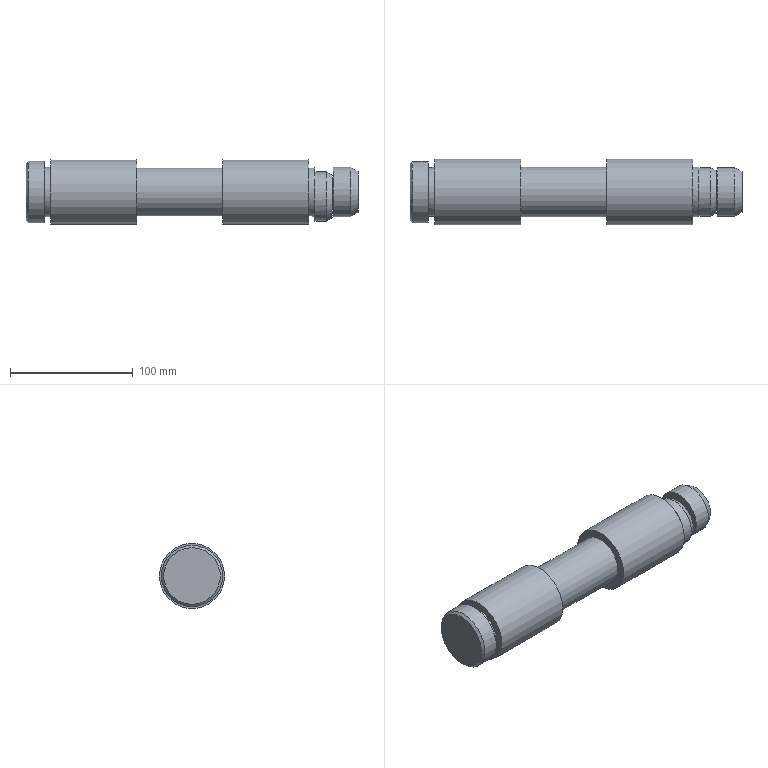Part | NX | features solid 2 | 1 solid | 33 faces | box 270 x 53 x 53 mm | volume 475072 mm3 | plane 14 | cylinder 12 | cone 7 | commonest cylinder face diameters 40 x5 53 x2 16 x1 16.2 x1 20 x1 27 x1
STEP:
#1=CARTESIAN_POINT('',(-925.,645.,-195.));
#2=VERTEX_POINT('',#1);
#3=CARTESIAN_POINT('',(-925.,625.,-195.));
#4=DIRECTION('',(1.,0.,0.));
#5=DIRECTION('',(0.,1.,0.));
#6=AXIS2_PLACEMENT_3D('',#3,#4,#5);
#7=CIRCLE('',#6,20.);
#8=EDGE_CURVE('',#2,#2,#7,.T.);
#9=ORIENTED_EDGE('',*,*,#8,.T.);
#10=EDGE_LOOP('',(#9));
#11=FACE_BOUND('',#10,.T.);
#12=CARTESIAN_POINT('',(-920.001,644.919,-196.8));
#13=VERTEX_POINT('',#12);
#14=CARTESIAN_POINT('',(-920.001,605.081,-196.8));
#15=VERTEX_POINT('',#14);
#16=CARTESIAN_POINT('',(-920.001,625.,-195.));
#17=DIRECTION('',(-1.,0.,0.));
#18=DIRECTION('',(0.,0.,1.));
#19=AXIS2_PLACEMENT_3D('',#16,#17,#18);
#20=CIRCLE('',#19,20.);
#21=EDGE_CURVE('',#13,#15,#20,.T.);
#22=ORIENTED_EDGE('',*,*,#21,.T.);
#23=CARTESIAN_POINT('',(-920.001,625.,-195.));
#24=DIRECTION('',(-1.,0.,0.));
#25=DIRECTION('',(0.,0.,1.));
#26=AXIS2_PLACEMENT_3D('',#23,#24,#25);
#27=CIRCLE('',#26,20.);
#28=EDGE_CURVE('',#15,#13,#27,.T.);
#29=ORIENTED_EDGE('',*,*,#28,.T.);
#30=EDGE_LOOP('',(#22,#29));
#31=FACE_BOUND('',#30,.T.);
#32=CARTESIAN_POINT('',(-1140.001,625.,-195.));
#33=DIRECTION('',(1.,0.,0.));
#34=DIRECTION('',(0.,0.,1.));
#35=AXIS2_PLACEMENT_3D('',#32,#33,#34);
#36=CYLINDRICAL_SURFACE('',#35,20.);
#37=ADVANCED_FACE('',(#11,#31),#36,.T.);
#38=CARTESIAN_POINT('',(-920.001,625.,-198.6));
#39=DIRECTION('',(-1.,0.,0.));
#40=DIRECTION('',(0.,-1.,0.));
#41=AXIS2_PLACEMENT_3D('',#38,#39,#40);
#42=CIRCLE('',#41,20.);
#43=EDGE_CURVE('',#15,#13,#42,.T.);
#44=ORIENTED_EDGE('',*,*,#43,.T.);
#45=ORIENTED_EDGE('',*,*,#28,.F.);
#46=EDGE_LOOP('',(#44,#45));
#47=FACE_BOUND('',#46,.T.);
#48=CARTESIAN_POINT('',(-920.001,625.,-195.));
#49=DIRECTION('',(1.,0.,0.));
#50=DIRECTION('',(0.,0.,1.));
#51=AXIS2_PLACEMENT_3D('',#48,#49,#50);
#52=PLANE('',#51);
#53=ADVANCED_FACE('',(#47),#52,.T.);
#54=CARTESIAN_POINT('',(-910.501,625.,-178.6));
#55=VERTEX_POINT('',#54);
#56=CARTESIAN_POINT('',(-910.501,625.,-198.6));
#57=DIRECTION('',(-1.,0.,0.));
#58=DIRECTION('',(0.,0.,1.));
#59=AXIS2_PLACEMENT_3D('',#56,#57,#58);
#60=CIRCLE('',#59,20.);
#61=EDGE_CURVE('',#55,#55,#60,.T.);
#62=ORIENTED_EDGE('',*,*,#61,.T.);
#63=EDGE_LOOP('',(#62));
#64=FACE_BOUND('',#63,.T.);
#65=CARTESIAN_POINT('',(-920.001,625.,-198.6));
#66=DIRECTION('',(-1.,0.,0.));
#67=DIRECTION('',(0.,0.,1.));
#68=AXIS2_PLACEMENT_3D('',#65,#66,#67);
#69=CIRCLE('',#68,20.);
#70=EDGE_CURVE('',#13,#15,#69,.T.);
#71=ORIENTED_EDGE('',*,*,#70,.F.);
#72=ORIENTED_EDGE('',*,*,#43,.F.);
#73=EDGE_LOOP('',(#71,#72));
#74=FACE_BOUND('',#73,.T.);
#75=CARTESIAN_POINT('',(-906.001,625.,-198.6));
#76=DIRECTION('',(-1.,0.,0.));
#77=DIRECTION('',(0.,0.,-1.));
#78=AXIS2_PLACEMENT_3D('',#75,#76,#77);
#79=CYLINDRICAL_SURFACE('',#78,20.);
#80=ADVANCED_FACE('',(#64,#74),#79,.T.);
#81=CARTESIAN_POINT('',(-906.001,622.282,-185.376));
#82=VERTEX_POINT('',#81);
#83=CARTESIAN_POINT('',(-906.001,627.718,-185.376));
#84=VERTEX_POINT('',#83);
#85=CARTESIAN_POINT('',(-906.001,625.,-195.));
#86=DIRECTION('',(-1.,0.,0.));
#87=DIRECTION('',(0.,1.,0.));
#88=AXIS2_PLACEMENT_3D('',#85,#86,#87);
#89=CIRCLE('',#88,10.);
#90=EDGE_CURVE('',#82,#84,#89,.T.);
#91=ORIENTED_EDGE('',*,*,#90,.T.);
#92=CARTESIAN_POINT('',(-906.001,625.,-198.6));
#93=DIRECTION('',(-1.,0.,0.));
#94=DIRECTION('',(0.,0.,1.));
#95=AXIS2_PLACEMENT_3D('',#92,#93,#94);
#96=CIRCLE('',#95,13.5);
#97=EDGE_CURVE('',#84,#82,#96,.T.);
#98=ORIENTED_EDGE('',*,*,#97,.T.);
#99=EDGE_LOOP('',(#91,#98));
#100=FACE_BOUND('',#99,.T.);
#101=CARTESIAN_POINT('',(-906.001,625.,-181.198));
#102=VERTEX_POINT('',#101);
#103=CARTESIAN_POINT('',(-906.001,625.,-198.6));
#104=DIRECTION('',(1.,0.,0.));
#105=DIRECTION('',(0.,0.,1.));
#106=AXIS2_PLACEMENT_3D('',#103,#104,#105);
#107=CIRCLE('',#106,17.402);
#108=EDGE_CURVE('',#102,#102,#107,.T.);
#109=ORIENTED_EDGE('',*,*,#108,.T.);
#110=EDGE_LOOP('',(#109));
#111=FACE_BOUND('',#110,.T.);
#112=CARTESIAN_POINT('',(-906.001,625.,-198.6));
#113=DIRECTION('',(-1.,0.,0.));
#114=DIRECTION('',(0.,0.,-1.));
#115=AXIS2_PLACEMENT_3D('',#112,#113,#114);
#116=PLANE('',#115);
#117=ADVANCED_FACE('',(#100,#111),#116,.F.);
#118=ORIENTED_EDGE('',*,*,#70,.T.);
#119=ORIENTED_EDGE('',*,*,#21,.F.);
#120=EDGE_LOOP('',(#118,#119));
#121=FACE_BOUND('',#120,.T.);
#122=CARTESIAN_POINT('',(-920.001,625.,-198.6));
#123=DIRECTION('',(-1.,0.,0.));
#124=DIRECTION('',(0.,0.,-1.));
#125=AXIS2_PLACEMENT_3D('',#122,#123,#124);
#126=PLANE('',#125);
#127=ADVANCED_FACE('',(#121),#126,.T.);
#128=ORIENTED_EDGE('',*,*,#108,.F.);
#129=EDGE_LOOP('',(#128));
#130=FACE_BOUND('',#129,.T.);
#131=ORIENTED_EDGE('',*,*,#61,.F.);
#132=EDGE_LOOP('',(#131));
#133=FACE_BOUND('',#132,.T.);
#134=CARTESIAN_POINT('',(-910.501,625.,-198.6));
#135=DIRECTION('',(-1.,0.,0.));
#136=DIRECTION('',(0.,0.,-1.));
#137=AXIS2_PLACEMENT_3D('',#134,#135,#136);
#138=CONICAL_SURFACE('',#137,20.,0.5236);
#139=ADVANCED_FACE('',(#130,#133),#138,.T.);
#140=CARTESIAN_POINT('',(-919.201,622.282,-185.376));
#141=VERTEX_POINT('',#140);
#142=CARTESIAN_POINT('',(-912.601,622.282,-185.376));
#143=DIRECTION('',(1.,0.,0.));
#144=VECTOR('',#143,1000.);
#145=LINE('',#142,#144);
#146=EDGE_CURVE('',#141,#82,#145,.T.);
#147=ORIENTED_EDGE('',*,*,#146,.T.);
#148=ORIENTED_EDGE('',*,*,#97,.F.);
#149=CARTESIAN_POINT('',(-919.201,627.718,-185.376));
#150=VERTEX_POINT('',#149);
#151=CARTESIAN_POINT('',(-912.601,627.718,-185.376));
#152=DIRECTION('',(-1.,0.,0.));
#153=VECTOR('',#152,1000.);
#154=LINE('',#151,#153);
#155=EDGE_CURVE('',#84,#150,#154,.T.);
#156=ORIENTED_EDGE('',*,*,#155,.T.);
#157=CARTESIAN_POINT('',(-919.201,625.,-198.6));
#158=DIRECTION('',(-1.,0.,0.));
#159=DIRECTION('',(0.,0.,1.));
#160=AXIS2_PLACEMENT_3D('',#157,#158,#159);
#161=CIRCLE('',#160,13.5);
#162=EDGE_CURVE('',#150,#141,#161,.T.);
#163=ORIENTED_EDGE('',*,*,#162,.T.);
#164=EDGE_LOOP('',(#147,#148,#156,#163));
#165=FACE_BOUND('',#164,.T.);
#166=CARTESIAN_POINT('',(-906.001,625.,-198.6));
#167=DIRECTION('',(-1.,0.,0.));
#168=DIRECTION('',(0.,0.,-1.));
#169=AXIS2_PLACEMENT_3D('',#166,#167,#168);
#170=CYLINDRICAL_SURFACE('',#169,13.5);
#171=ADVANCED_FACE('',(#165),#170,.F.);
#172=CARTESIAN_POINT('',(-920.001,610.7,-198.6));
#173=VERTEX_POINT('',#172);
#174=CARTESIAN_POINT('',(-920.001,625.,-198.6));
#175=DIRECTION('',(1.,0.,0.));
#176=DIRECTION('',(0.,-1.,0.));
#177=AXIS2_PLACEMENT_3D('',#174,#175,#176);
#178=CIRCLE('',#177,14.3);
#179=EDGE_CURVE('',#173,#173,#178,.T.);
#180=ORIENTED_EDGE('',*,*,#179,.F.);
#181=EDGE_LOOP('',(#180));
#182=FACE_BOUND('',#181,.T.);
#183=ORIENTED_EDGE('',*,*,#162,.F.);
#184=CARTESIAN_POINT('',(-919.201,622.282,-185.376));
#185=CARTESIAN_POINT('',(-919.334,624.058,-184.875));
#186=CARTESIAN_POINT('',(-919.334,625.942,-184.875));
#187=CARTESIAN_POINT('',(-919.201,627.718,-185.376));
#188=B_SPLINE_CURVE_WITH_KNOTS('',3,(#184,#185,#186,#187),.UNSPECIFIED.,.F.,.F.,(4,4),(0.,0.005472),.UNSPECIFIED.);
#189=EDGE_CURVE('',#141,#150,#188,.T.);
#190=ORIENTED_EDGE('',*,*,#189,.F.);
#191=EDGE_LOOP('',(#183,#190));
#192=FACE_BOUND('',#191,.T.);
#193=CARTESIAN_POINT('',(-919.201,625.,-198.6));
#194=DIRECTION('',(-1.,0.,0.));
#195=DIRECTION('',(0.,0.,-1.));
#196=AXIS2_PLACEMENT_3D('',#193,#194,#195);
#197=CONICAL_SURFACE('',#196,13.5,0.7854);
#198=ADVANCED_FACE('',(#182,#192),#197,.F.);
#199=CARTESIAN_POINT('',(-920.001,625.,-185.));
#200=VERTEX_POINT('',#199);
#201=CARTESIAN_POINT('',(-920.001,625.,-195.));
#202=DIRECTION('',(1.,0.,0.));
#203=DIRECTION('',(0.,0.,1.));
#204=AXIS2_PLACEMENT_3D('',#201,#202,#203);
#205=CIRCLE('',#204,10.);
#206=EDGE_CURVE('',#200,#200,#205,.T.);
#207=ORIENTED_EDGE('',*,*,#206,.T.);
#208=EDGE_LOOP('',(#207));
#209=FACE_BOUND('',#208,.T.);
#210=CARTESIAN_POINT('',(-905.001,635.,-195.));
#211=VERTEX_POINT('',#210);
#212=CARTESIAN_POINT('',(-905.001,625.,-195.));
#213=DIRECTION('',(-1.,0.,0.));
#214=DIRECTION('',(0.,1.,0.));
#215=AXIS2_PLACEMENT_3D('',#212,#213,#214);
#216=CIRCLE('',#215,10.);
#217=EDGE_CURVE('',#211,#211,#216,.T.);
#218=ORIENTED_EDGE('',*,*,#217,.T.);
#219=EDGE_LOOP('',(#218));
#220=FACE_BOUND('',#219,.T.);
#221=ORIENTED_EDGE('',*,*,#146,.F.);
#222=ORIENTED_EDGE('',*,*,#189,.T.);
#223=ORIENTED_EDGE('',*,*,#155,.F.);
#224=ORIENTED_EDGE('',*,*,#90,.F.);
#225=EDGE_LOOP('',(#221,#222,#223,#224));
#226=FACE_BOUND('',#225,.T.);
#227=CARTESIAN_POINT('',(-920.001,625.,-195.));
#228=DIRECTION('',(1.,0.,0.));
#229=DIRECTION('',(0.,0.,1.));
#230=AXIS2_PLACEMENT_3D('',#227,#228,#229);
#231=CYLINDRICAL_SURFACE('',#230,10.);
#232=ADVANCED_FACE('',(#209,#220,#226),#231,.T.);
#233=ORIENTED_EDGE('',*,*,#179,.T.);
#234=EDGE_LOOP('',(#233));
#235=FACE_BOUND('',#234,.T.);
#236=ORIENTED_EDGE('',*,*,#206,.F.);
#237=EDGE_LOOP('',(#236));
#238=FACE_BOUND('',#237,.T.);
#239=CARTESIAN_POINT('',(-920.001,625.,-195.));
#240=DIRECTION('',(1.,0.,0.));
#241=DIRECTION('',(0.,0.,1.));
#242=AXIS2_PLACEMENT_3D('',#239,#240,#241);
#243=PLANE('',#242);
#244=ADVANCED_FACE('',(#235,#238),#243,.T.);
#245=ORIENTED_EDGE('',*,*,#8,.F.);
#246=EDGE_LOOP('',(#245));
#247=FACE_BOUND('',#246,.T.);
#248=CARTESIAN_POINT('',(-925.,651.5,-195.));
#249=VERTEX_POINT('',#248);
#250=CARTESIAN_POINT('',(-925.,625.,-195.));
#251=DIRECTION('',(1.,0.,0.));
#252=DIRECTION('',(0.,1.,0.));
#253=AXIS2_PLACEMENT_3D('',#250,#251,#252);
#254=CIRCLE('',#253,26.5);
#255=EDGE_CURVE('',#249,#249,#254,.T.);
#256=ORIENTED_EDGE('',*,*,#255,.T.);
#257=EDGE_LOOP('',(#256));
#258=FACE_BOUND('',#257,.T.);
#259=CARTESIAN_POINT('',(-925.,625.,-195.));
#260=DIRECTION('',(-1.,0.,0.));
#261=DIRECTION('',(0.,0.,1.));
#262=AXIS2_PLACEMENT_3D('',#259,#260,#261);
#263=PLANE('',#262);
#264=ADVANCED_FACE('',(#247,#258),#263,.F.);
#265=CARTESIAN_POINT('',(-995.,645.,-195.));
#266=VERTEX_POINT('',#265);
#267=CARTESIAN_POINT('',(-995.,625.,-195.));
#268=DIRECTION('',(-1.,0.,0.));
#269=DIRECTION('',(0.,1.,0.));
#270=AXIS2_PLACEMENT_3D('',#267,#268,#269);
#271=CIRCLE('',#270,20.);
#272=EDGE_CURVE('',#266,#266,#271,.T.);
#273=ORIENTED_EDGE('',*,*,#272,.F.);
#274=EDGE_LOOP('',(#273));
#275=FACE_BOUND('',#274,.T.);
#276=CARTESIAN_POINT('',(-995.,651.5,-195.));
#277=VERTEX_POINT('',#276);
#278=CARTESIAN_POINT('',(-995.,625.,-195.));
#279=DIRECTION('',(1.,0.,0.));
#280=DIRECTION('',(0.,1.,0.));
#281=AXIS2_PLACEMENT_3D('',#278,#279,#280);
#282=CIRCLE('',#281,26.5);
#283=EDGE_CURVE('',#277,#277,#282,.T.);
#284=ORIENTED_EDGE('',*,*,#283,.F.);
#285=EDGE_LOOP('',(#284));
#286=FACE_BOUND('',#285,.T.);
#287=CARTESIAN_POINT('',(-995.,625.,-195.));
#288=DIRECTION('',(-1.,0.,0.));
#289=DIRECTION('',(0.,0.,1.));
#290=AXIS2_PLACEMENT_3D('',#287,#288,#289);
#291=PLANE('',#290);
#292=ADVANCED_FACE('',(#275,#286),#291,.T.);
#293=ORIENTED_EDGE('',*,*,#255,.F.);
#294=EDGE_LOOP('',(#293));
#295=FACE_BOUND('',#294,.T.);
#296=ORIENTED_EDGE('',*,*,#283,.T.);
#297=EDGE_LOOP('',(#296));
#298=FACE_BOUND('',#297,.T.);
#299=CARTESIAN_POINT('',(-995.,625.,-195.));
#300=DIRECTION('',(1.,0.,0.));
#301=DIRECTION('',(0.,0.,-1.));
#302=AXIS2_PLACEMENT_3D('',#299,#300,#301);
#303=CYLINDRICAL_SURFACE('',#302,26.5);
#304=ADVANCED_FACE('',(#295,#298),#303,.T.);
#305=CARTESIAN_POINT('',(-1155.001,625.,-218.));
#306=VERTEX_POINT('',#305);
#307=CARTESIAN_POINT('',(-1155.001,625.,-195.));
#308=DIRECTION('',(-1.,0.,0.));
#309=DIRECTION('',(0.,0.,-1.));
#310=AXIS2_PLACEMENT_3D('',#307,#308,#309);
#311=CIRCLE('',#310,23.);
#312=EDGE_CURVE('',#306,#306,#311,.T.);
#313=ORIENTED_EDGE('',*,*,#312,.T.);
#314=EDGE_LOOP('',(#313));
#315=FACE_BOUND('',#314,.T.);
#316=CARTESIAN_POINT('',(-1155.001,625.,-195.));
#317=DIRECTION('',(-1.,0.,0.));
#318=DIRECTION('',(0.,0.,-1.));
#319=AXIS2_PLACEMENT_3D('',#316,#317,#318);
#320=PLANE('',#319);
#321=ADVANCED_FACE('',(#315),#320,.T.);
#322=CARTESIAN_POINT('',(-1153.001,625.,-220.));
#323=VERTEX_POINT('',#322);
#324=CARTESIAN_POINT('',(-1153.001,625.,-195.));
#325=DIRECTION('',(1.,0.,0.));
#326=DIRECTION('',(0.,0.,-1.));
#327=AXIS2_PLACEMENT_3D('',#324,#325,#326);
#328=CIRCLE('',#327,25.);
#329=EDGE_CURVE('',#323,#323,#328,.T.);
#330=ORIENTED_EDGE('',*,*,#329,.F.);
#331=EDGE_LOOP('',(#330));
#332=FACE_BOUND('',#331,.T.);
#333=ORIENTED_EDGE('',*,*,#312,.F.);
#334=EDGE_LOOP('',(#333));
#335=FACE_BOUND('',#334,.T.);
#336=CARTESIAN_POINT('',(-1155.001,625.,-195.));
#337=DIRECTION('',(1.,0.,0.));
#338=DIRECTION('',(0.,0.,-1.));
#339=AXIS2_PLACEMENT_3D('',#336,#337,#338);
#340=CONICAL_SURFACE('',#339,23.,0.7854);
#341=ADVANCED_FACE('',(#332,#335),#340,.T.);
#342=ORIENTED_EDGE('',*,*,#329,.T.);
#343=EDGE_LOOP('',(#342));
#344=FACE_BOUND('',#343,.T.);
#345=CARTESIAN_POINT('',(-1140.001,625.,-170.));
#346=VERTEX_POINT('',#345);
#347=CARTESIAN_POINT('',(-1140.001,625.,-195.));
#348=DIRECTION('',(-1.,0.,0.));
#349=DIRECTION('',(0.,0.,1.));
#350=AXIS2_PLACEMENT_3D('',#347,#348,#349);
#351=CIRCLE('',#350,25.);
#352=EDGE_CURVE('',#346,#346,#351,.T.);
#353=ORIENTED_EDGE('',*,*,#352,.T.);
#354=EDGE_LOOP('',(#353));
#355=FACE_BOUND('',#354,.T.);
#356=CARTESIAN_POINT('',(-1140.001,625.,-195.));
#357=DIRECTION('',(-1.,0.,0.));
#358=DIRECTION('',(0.,0.,-1.));
#359=AXIS2_PLACEMENT_3D('',#356,#357,#358);
#360=CYLINDRICAL_SURFACE('',#359,25.);
#361=ADVANCED_FACE('',(#344,#355),#360,.T.);
#362=CARTESIAN_POINT('',(-1140.001,625.,-175.));
#363=VERTEX_POINT('',#362);
#364=CARTESIAN_POINT('',(-1140.001,625.,-195.));
#365=DIRECTION('',(-1.,0.,0.));
#366=DIRECTION('',(0.,0.,1.));
#367=AXIS2_PLACEMENT_3D('',#364,#365,#366);
#368=CIRCLE('',#367,20.);
#369=EDGE_CURVE('',#363,#363,#368,.T.);
#370=ORIENTED_EDGE('',*,*,#369,.T.);
#371=EDGE_LOOP('',(#370));
#372=FACE_BOUND('',#371,.T.);
#373=ORIENTED_EDGE('',*,*,#352,.F.);
#374=EDGE_LOOP('',(#373));
#375=FACE_BOUND('',#374,.T.);
#376=CARTESIAN_POINT('',(-1140.001,625.,-195.));
#377=DIRECTION('',(1.,0.,0.));
#378=DIRECTION('',(0.,0.,1.));
#379=AXIS2_PLACEMENT_3D('',#376,#377,#378);
#380=PLANE('',#379);
#381=ADVANCED_FACE('',(#372,#375),#380,.T.);
#382=CARTESIAN_POINT('',(-1135.001,645.,-195.));
#383=VERTEX_POINT('',#382);
#384=CARTESIAN_POINT('',(-1135.001,625.,-195.));
#385=DIRECTION('',(1.,0.,0.));
#386=DIRECTION('',(0.,1.,0.));
#387=AXIS2_PLACEMENT_3D('',#384,#385,#386);
#388=CIRCLE('',#387,20.);
#389=EDGE_CURVE('',#383,#383,#388,.T.);
#390=ORIENTED_EDGE('',*,*,#389,.F.);
#391=EDGE_LOOP('',(#390));
#392=FACE_BOUND('',#391,.T.);
#393=ORIENTED_EDGE('',*,*,#369,.F.);
#394=EDGE_LOOP('',(#393));
#395=FACE_BOUND('',#394,.T.);
#396=CARTESIAN_POINT('',(-1140.001,625.,-195.));
#397=DIRECTION('',(1.,0.,0.));
#398=DIRECTION('',(0.,0.,1.));
#399=AXIS2_PLACEMENT_3D('',#396,#397,#398);
#400=CYLINDRICAL_SURFACE('',#399,20.);
#401=ADVANCED_FACE('',(#392,#395),#400,.T.);
#402=ORIENTED_EDGE('',*,*,#389,.T.);
#403=EDGE_LOOP('',(#402));
#404=FACE_BOUND('',#403,.T.);
#405=CARTESIAN_POINT('',(-1135.001,651.5,-195.));
#406=VERTEX_POINT('',#405);
#407=CARTESIAN_POINT('',(-1135.001,625.,-195.));
#408=DIRECTION('',(1.,0.,0.));
#409=DIRECTION('',(0.,1.,0.));
#410=AXIS2_PLACEMENT_3D('',#407,#408,#409);
#411=CIRCLE('',#410,26.5);
#412=EDGE_CURVE('',#406,#406,#411,.T.);
#413=ORIENTED_EDGE('',*,*,#412,.F.);
#414=EDGE_LOOP('',(#413));
#415=FACE_BOUND('',#414,.T.);
#416=CARTESIAN_POINT('',(-1135.001,625.,-195.));
#417=DIRECTION('',(-1.,0.,0.));
#418=DIRECTION('',(0.,0.,1.));
#419=AXIS2_PLACEMENT_3D('',#416,#417,#418);
#420=PLANE('',#419);
#421=ADVANCED_FACE('',(#404,#415),#420,.T.);
#422=CARTESIAN_POINT('',(-1065.001,651.5,-195.));
#423=VERTEX_POINT('',#422);
#424=CARTESIAN_POINT('',(-1065.001,625.,-195.));
#425=DIRECTION('',(1.,0.,0.));
#426=DIRECTION('',(0.,1.,0.));
#427=AXIS2_PLACEMENT_3D('',#424,#425,#426);
#428=CIRCLE('',#427,26.5);
#429=EDGE_CURVE('',#423,#423,#428,.T.);
#430=ORIENTED_EDGE('',*,*,#429,.F.);
#431=EDGE_LOOP('',(#430));
#432=FACE_BOUND('',#431,.T.);
#433=ORIENTED_EDGE('',*,*,#412,.T.);
#434=EDGE_LOOP('',(#433));
#435=FACE_BOUND('',#434,.T.);
#436=CARTESIAN_POINT('',(-1135.001,625.,-195.));
#437=DIRECTION('',(1.,0.,0.));
#438=DIRECTION('',(0.,0.,-1.));
#439=AXIS2_PLACEMENT_3D('',#436,#437,#438);
#440=CYLINDRICAL_SURFACE('',#439,26.5);
#441=ADVANCED_FACE('',(#432,#435),#440,.T.);
#442=CARTESIAN_POINT('',(-1065.001,645.,-195.));
#443=VERTEX_POINT('',#442);
#444=CARTESIAN_POINT('',(-1065.001,625.,-195.));
#445=DIRECTION('',(-1.,0.,0.));
#446=DIRECTION('',(0.,1.,0.));
#447=AXIS2_PLACEMENT_3D('',#444,#445,#446);
#448=CIRCLE('',#447,20.);
#449=EDGE_CURVE('',#443,#443,#448,.T.);
#450=ORIENTED_EDGE('',*,*,#449,.T.);
#451=EDGE_LOOP('',(#450));
#452=FACE_BOUND('',#451,.T.);
#453=ORIENTED_EDGE('',*,*,#429,.T.);
#454=EDGE_LOOP('',(#453));
#455=FACE_BOUND('',#454,.T.);
#456=CARTESIAN_POINT('',(-1065.001,625.,-195.));
#457=DIRECTION('',(-1.,0.,0.));
#458=DIRECTION('',(0.,0.,1.));
#459=AXIS2_PLACEMENT_3D('',#456,#457,#458);
#460=PLANE('',#459);
#461=ADVANCED_FACE('',(#452,#455),#460,.F.);
#462=ORIENTED_EDGE('',*,*,#272,.T.);
#463=EDGE_LOOP('',(#462));
#464=FACE_BOUND('',#463,.T.);
#465=ORIENTED_EDGE('',*,*,#449,.F.);
#466=EDGE_LOOP('',(#465));
#467=FACE_BOUND('',#466,.T.);
#468=CARTESIAN_POINT('',(-1140.001,625.,-195.));
#469=DIRECTION('',(1.,0.,0.));
#470=DIRECTION('',(0.,0.,1.));
#471=AXIS2_PLACEMENT_3D('',#468,#469,#470);
#472=CYLINDRICAL_SURFACE('',#471,20.);
#473=ADVANCED_FACE('',(#464,#467),#472,.T.);
#474=CARTESIAN_POINT('',(-891.001,625.,-175.));
#475=VERTEX_POINT('',#474);
#476=CARTESIAN_POINT('',(-891.001,625.,-195.));
#477=DIRECTION('',(-1.,0.,0.));
#478=DIRECTION('',(0.,0.,1.));
#479=AXIS2_PLACEMENT_3D('',#476,#477,#478);
#480=CIRCLE('',#479,20.);
#481=EDGE_CURVE('',#475,#475,#480,.T.);
#482=ORIENTED_EDGE('',*,*,#481,.T.);
#483=EDGE_LOOP('',(#482));
#484=FACE_BOUND('',#483,.T.);
#485=CARTESIAN_POINT('',(-905.001,625.,-175.));
#486=VERTEX_POINT('',#485);
#487=CARTESIAN_POINT('',(-905.001,625.,-195.));
#488=DIRECTION('',(-1.,0.,0.));
#489=DIRECTION('',(0.,0.,1.));
#490=AXIS2_PLACEMENT_3D('',#487,#488,#489);
#491=CIRCLE('',#490,20.);
#492=EDGE_CURVE('',#486,#486,#491,.T.);
#493=ORIENTED_EDGE('',*,*,#492,.F.);
#494=EDGE_LOOP('',(#493));
#495=FACE_BOUND('',#494,.T.);
#496=CARTESIAN_POINT('',(-885.001,625.,-195.));
#497=DIRECTION('',(-1.,0.,0.));
#498=DIRECTION('',(0.,0.,-1.));
#499=AXIS2_PLACEMENT_3D('',#496,#497,#498);
#500=CYLINDRICAL_SURFACE('',#499,20.);
#501=ADVANCED_FACE('',(#484,#495),#500,.T.);
#502=CARTESIAN_POINT('',(-885.001,625.,-182.9));
#503=VERTEX_POINT('',#502);
#504=CARTESIAN_POINT('',(-885.001,625.,-195.));
#505=DIRECTION('',(-1.,0.,0.));
#506=DIRECTION('',(0.,0.,1.));
#507=AXIS2_PLACEMENT_3D('',#504,#505,#506);
#508=CIRCLE('',#507,12.1);
#509=EDGE_CURVE('',#503,#503,#508,.T.);
#510=ORIENTED_EDGE('',*,*,#509,.T.);
#511=EDGE_LOOP('',(#510));
#512=FACE_BOUND('',#511,.T.);
#513=CARTESIAN_POINT('',(-885.001,625.,-178.464));
#514=VERTEX_POINT('',#513);
#515=CARTESIAN_POINT('',(-885.001,625.,-195.));
#516=DIRECTION('',(1.,0.,0.));
#517=DIRECTION('',(0.,0.,1.));
#518=AXIS2_PLACEMENT_3D('',#515,#516,#517);
#519=CIRCLE('',#518,16.536);
#520=EDGE_CURVE('',#514,#514,#519,.T.);
#521=ORIENTED_EDGE('',*,*,#520,.T.);
#522=EDGE_LOOP('',(#521));
#523=FACE_BOUND('',#522,.T.);
#524=CARTESIAN_POINT('',(-885.001,625.,-195.));
#525=DIRECTION('',(-1.,0.,0.));
#526=DIRECTION('',(0.,0.,-1.));
#527=AXIS2_PLACEMENT_3D('',#524,#525,#526);
#528=PLANE('',#527);
#529=ADVANCED_FACE('',(#512,#523),#528,.F.);
#530=ORIENTED_EDGE('',*,*,#217,.F.);
#531=EDGE_LOOP('',(#530));
#532=FACE_BOUND('',#531,.T.);
#533=ORIENTED_EDGE('',*,*,#492,.T.);
#534=EDGE_LOOP('',(#533));
#535=FACE_BOUND('',#534,.T.);
#536=CARTESIAN_POINT('',(-905.001,625.,-195.));
#537=DIRECTION('',(-1.,0.,0.));
#538=DIRECTION('',(0.,0.,-1.));
#539=AXIS2_PLACEMENT_3D('',#536,#537,#538);
#540=PLANE('',#539);
#541=ADVANCED_FACE('',(#532,#535),#540,.T.);
#542=CARTESIAN_POINT('',(-904.201,625.,-186.9));
#543=VERTEX_POINT('',#542);
#544=CARTESIAN_POINT('',(-904.201,625.,-195.));
#545=DIRECTION('',(-1.,0.,0.));
#546=DIRECTION('',(0.,0.,1.));
#547=AXIS2_PLACEMENT_3D('',#544,#545,#546);
#548=CIRCLE('',#547,8.1);
#549=EDGE_CURVE('',#543,#543,#548,.T.);
#550=ORIENTED_EDGE('',*,*,#549,.T.);
#551=EDGE_LOOP('',(#550));
#552=FACE_BOUND('',#551,.T.);
#553=CARTESIAN_POINT('',(-889.001,625.,-186.9));
#554=VERTEX_POINT('',#553);
#555=CARTESIAN_POINT('',(-889.001,625.,-195.));
#556=DIRECTION('',(1.,0.,0.));
#557=DIRECTION('',(0.,0.,1.));
#558=AXIS2_PLACEMENT_3D('',#555,#556,#557);
#559=CIRCLE('',#558,8.1);
#560=EDGE_CURVE('',#554,#554,#559,.T.);
#561=ORIENTED_EDGE('',*,*,#560,.T.);
#562=EDGE_LOOP('',(#561));
#563=FACE_BOUND('',#562,.T.);
#564=CARTESIAN_POINT('',(-885.001,625.,-195.));
#565=DIRECTION('',(-1.,0.,0.));
#566=DIRECTION('',(0.,0.,-1.));
#567=AXIS2_PLACEMENT_3D('',#564,#565,#566);
#568=CYLINDRICAL_SURFACE('',#567,8.1);
#569=ADVANCED_FACE('',(#552,#563),#568,.F.);
#570=ORIENTED_EDGE('',*,*,#520,.F.);
#571=EDGE_LOOP('',(#570));
#572=FACE_BOUND('',#571,.T.);
#573=ORIENTED_EDGE('',*,*,#481,.F.);
#574=EDGE_LOOP('',(#573));
#575=FACE_BOUND('',#574,.T.);
#576=CARTESIAN_POINT('',(-891.001,625.,-195.));
#577=DIRECTION('',(-1.,0.,0.));
#578=DIRECTION('',(0.,0.,-1.));
#579=AXIS2_PLACEMENT_3D('',#576,#577,#578);
#580=CONICAL_SURFACE('',#579,20.,0.5236);
#581=ADVANCED_FACE('',(#572,#575),#580,.T.);
#582=ORIENTED_EDGE('',*,*,#560,.F.);
#583=EDGE_LOOP('',(#582));
#584=FACE_BOUND('',#583,.T.);
#585=ORIENTED_EDGE('',*,*,#509,.F.);
#586=EDGE_LOOP('',(#585));
#587=FACE_BOUND('',#586,.T.);
#588=CARTESIAN_POINT('',(-885.001,625.,-195.));
#589=DIRECTION('',(1.,0.,0.));
#590=DIRECTION('',(0.,0.,1.));
#591=AXIS2_PLACEMENT_3D('',#588,#589,#590);
#592=CONICAL_SURFACE('',#591,12.1,0.7854);
#593=ADVANCED_FACE('',(#584,#587),#592,.F.);
#594=CARTESIAN_POINT('',(-905.001,616.1,-195.));
#595=VERTEX_POINT('',#594);
#596=CARTESIAN_POINT('',(-905.001,625.,-195.));
#597=DIRECTION('',(1.,0.,0.));
#598=DIRECTION('',(0.,-1.,0.));
#599=AXIS2_PLACEMENT_3D('',#596,#597,#598);
#600=CIRCLE('',#599,8.9);
#601=EDGE_CURVE('',#595,#595,#600,.T.);
#602=ORIENTED_EDGE('',*,*,#601,.F.);
#603=EDGE_LOOP('',(#602));
#604=FACE_BOUND('',#603,.T.);
#605=ORIENTED_EDGE('',*,*,#549,.F.);
#606=EDGE_LOOP('',(#605));
#607=FACE_BOUND('',#606,.T.);
#608=CARTESIAN_POINT('',(-904.201,625.,-195.));
#609=DIRECTION('',(-1.,0.,0.));
#610=DIRECTION('',(0.,0.,-1.));
#611=AXIS2_PLACEMENT_3D('',#608,#609,#610);
#612=CONICAL_SURFACE('',#611,8.1,0.7854);
#613=ADVANCED_FACE('',(#604,#607),#612,.F.);
#614=CARTESIAN_POINT('',(-885.001,625.,-191.));
#615=VERTEX_POINT('',#614);
#616=CARTESIAN_POINT('',(-885.001,625.,-195.));
#617=DIRECTION('',(1.,0.,0.));
#618=DIRECTION('',(0.,0.,1.));
#619=AXIS2_PLACEMENT_3D('',#616,#617,#618);
#620=CIRCLE('',#619,4.);
#621=EDGE_CURVE('',#615,#615,#620,.T.);
#622=ORIENTED_EDGE('',*,*,#621,.T.);
#623=EDGE_LOOP('',(#622));
#624=FACE_BOUND('',#623,.T.);
#625=CARTESIAN_POINT('',(-885.001,625.,-195.));
#626=DIRECTION('',(1.,0.,0.));
#627=DIRECTION('',(0.,0.,1.));
#628=AXIS2_PLACEMENT_3D('',#625,#626,#627);
#629=PLANE('',#628);
#630=ADVANCED_FACE('',(#624),#629,.T.);
#631=CARTESIAN_POINT('',(-889.001,625.,-187.));
#632=VERTEX_POINT('',#631);
#633=CARTESIAN_POINT('',(-889.001,625.,-195.));
#634=DIRECTION('',(-1.,0.,0.));
#635=DIRECTION('',(0.,0.,1.));
#636=AXIS2_PLACEMENT_3D('',#633,#634,#635);
#637=CIRCLE('',#636,8.);
#638=EDGE_CURVE('',#632,#632,#637,.T.);
#639=ORIENTED_EDGE('',*,*,#638,.F.);
#640=EDGE_LOOP('',(#639));
#641=FACE_BOUND('',#640,.T.);
#642=ORIENTED_EDGE('',*,*,#621,.F.);
#643=EDGE_LOOP('',(#642));
#644=FACE_BOUND('',#643,.T.);
#645=CARTESIAN_POINT('',(-885.001,625.,-195.));
#646=DIRECTION('',(-1.,0.,0.));
#647=DIRECTION('',(0.,0.,1.));
#648=AXIS2_PLACEMENT_3D('',#645,#646,#647);
#649=CONICAL_SURFACE('',#648,4.,0.7854);
#650=ADVANCED_FACE('',(#641,#644),#649,.T.);
#651=ORIENTED_EDGE('',*,*,#638,.T.);
#652=EDGE_LOOP('',(#651));
#653=FACE_BOUND('',#652,.T.);
#654=CARTESIAN_POINT('',(-905.001,625.,-187.));
#655=VERTEX_POINT('',#654);
#656=CARTESIAN_POINT('',(-905.001,625.,-195.));
#657=DIRECTION('',(1.,0.,0.));
#658=DIRECTION('',(0.,0.,1.));
#659=AXIS2_PLACEMENT_3D('',#656,#657,#658);
#660=CIRCLE('',#659,8.);
#661=EDGE_CURVE('',#655,#655,#660,.T.);
#662=ORIENTED_EDGE('',*,*,#661,.T.);
#663=EDGE_LOOP('',(#662));
#664=FACE_BOUND('',#663,.T.);
#665=CARTESIAN_POINT('',(-905.001,625.,-195.));
#666=DIRECTION('',(1.,0.,0.));
#667=DIRECTION('',(0.,0.,1.));
#668=AXIS2_PLACEMENT_3D('',#665,#666,#667);
#669=CYLINDRICAL_SURFACE('',#668,8.);
#670=ADVANCED_FACE('',(#653,#664),#669,.T.);
#671=ORIENTED_EDGE('',*,*,#601,.T.);
#672=EDGE_LOOP('',(#671));
#673=FACE_BOUND('',#672,.T.);
#674=ORIENTED_EDGE('',*,*,#661,.F.);
#675=EDGE_LOOP('',(#674));
#676=FACE_BOUND('',#675,.T.);
#677=CARTESIAN_POINT('',(-905.001,625.,-195.));
#678=DIRECTION('',(1.,0.,0.));
#679=DIRECTION('',(0.,0.,1.));
#680=AXIS2_PLACEMENT_3D('',#677,#678,#679);
#681=PLANE('',#680);
#682=ADVANCED_FACE('',(#673,#676),#681,.T.);
#683=CLOSED_SHELL('',(#37,#53,#80,#117,#127,#139,#171,#198,#232,#244,#264,#292,#304,#321,#341,#361,#381,#401,#421,#441,#461,#473,#501,#529,#541,#569,#581,#593,#613,#630,#650,#670,#682));
#684=MANIFOLD_SOLID_BREP('',#683);
#685=(LENGTH_UNIT()NAMED_UNIT(*)SI_UNIT(.MILLI.,.METRE.));
#686=UNCERTAINTY_MEASURE_WITH_UNIT(LENGTH_MEASURE(0.0508),#685,'','');
#687=(NAMED_UNIT(*)PLANE_ANGLE_UNIT()SI_UNIT($,.RADIAN.));
#688=(NAMED_UNIT(*)SI_UNIT($,.STERADIAN.)SOLID_ANGLE_UNIT());
#689=(GEOMETRIC_REPRESENTATION_CONTEXT(3)GLOBAL_UNCERTAINTY_ASSIGNED_CONTEXT((#686))GLOBAL_UNIT_ASSIGNED_CONTEXT((#685,#687,#688))REPRESENTATION_CONTEXT('',''));
#690=ADVANCED_BREP_SHAPE_REPRESENTATION('',(#684),#689);